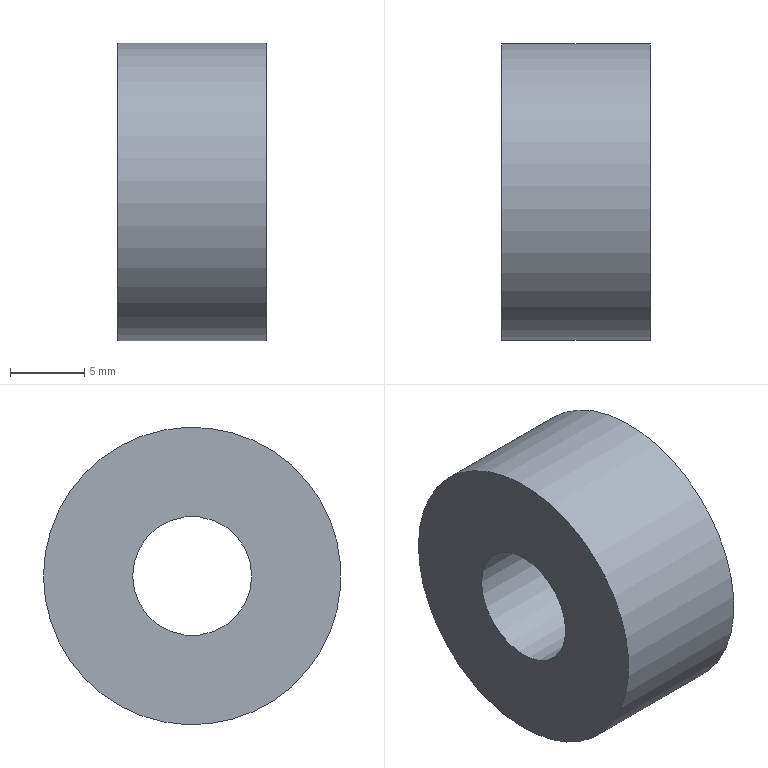Part | NX | features DATUM_CSYS 2, EXTRUDE 1, SKETCH 1 | 1 solid | 4 faces | box 10 x 20 x 20 mm | volume 2639 mm3 | cylinder 2 | plane 2 | commonest cylinder face diameters 8 x1 20 x1
STEP:
#1=CARTESIAN_POINT('',(10.,10.,0.));
#2=VERTEX_POINT('',#1);
#3=CARTESIAN_POINT('',(10.,0.,0.));
#4=DIRECTION('',(1.,0.,0.));
#5=DIRECTION('',(0.,1.,0.));
#6=AXIS2_PLACEMENT_3D('',#3,#4,#5);
#7=CIRCLE('',#6,10.);
#8=EDGE_CURVE('',#2,#2,#7,.T.);
#9=ORIENTED_EDGE('',*,*,#8,.F.);
#10=EDGE_LOOP('',(#9));
#11=FACE_BOUND('',#10,.T.);
#12=CARTESIAN_POINT('',(0.,10.,0.));
#13=VERTEX_POINT('',#12);
#14=CARTESIAN_POINT('',(0.,0.,0.));
#15=DIRECTION('',(1.,0.,0.));
#16=DIRECTION('',(0.,1.,0.));
#17=AXIS2_PLACEMENT_3D('',#14,#15,#16);
#18=CIRCLE('',#17,10.);
#19=EDGE_CURVE('',#13,#13,#18,.T.);
#20=ORIENTED_EDGE('',*,*,#19,.T.);
#21=EDGE_LOOP('',(#20));
#22=FACE_BOUND('',#21,.T.);
#23=CARTESIAN_POINT('',(10.,0.,0.));
#24=DIRECTION('',(-1.,0.,0.));
#25=DIRECTION('',(0.,0.,1.));
#26=AXIS2_PLACEMENT_3D('',#23,#24,#25);
#27=CYLINDRICAL_SURFACE('',#26,10.);
#28=ADVANCED_FACE('',(#11,#22),#27,.T.);
#29=CARTESIAN_POINT('',(10.,4.,0.));
#30=VERTEX_POINT('',#29);
#31=CARTESIAN_POINT('',(10.,0.,0.));
#32=DIRECTION('',(1.,0.,0.));
#33=DIRECTION('',(0.,1.,0.));
#34=AXIS2_PLACEMENT_3D('',#31,#32,#33);
#35=CIRCLE('',#34,4.);
#36=EDGE_CURVE('',#30,#30,#35,.T.);
#37=ORIENTED_EDGE('',*,*,#36,.T.);
#38=EDGE_LOOP('',(#37));
#39=FACE_BOUND('',#38,.T.);
#40=CARTESIAN_POINT('',(0.,4.,0.));
#41=VERTEX_POINT('',#40);
#42=CARTESIAN_POINT('',(0.,0.,0.));
#43=DIRECTION('',(1.,0.,0.));
#44=DIRECTION('',(0.,1.,0.));
#45=AXIS2_PLACEMENT_3D('',#42,#43,#44);
#46=CIRCLE('',#45,4.);
#47=EDGE_CURVE('',#41,#41,#46,.T.);
#48=ORIENTED_EDGE('',*,*,#47,.F.);
#49=EDGE_LOOP('',(#48));
#50=FACE_BOUND('',#49,.T.);
#51=CARTESIAN_POINT('',(10.,0.,0.));
#52=DIRECTION('',(-1.,0.,0.));
#53=DIRECTION('',(0.,0.,1.));
#54=AXIS2_PLACEMENT_3D('',#51,#52,#53);
#55=CYLINDRICAL_SURFACE('',#54,4.);
#56=ADVANCED_FACE('',(#39,#50),#55,.F.);
#57=ORIENTED_EDGE('',*,*,#8,.T.);
#58=EDGE_LOOP('',(#57));
#59=FACE_BOUND('',#58,.T.);
#60=ORIENTED_EDGE('',*,*,#36,.F.);
#61=EDGE_LOOP('',(#60));
#62=FACE_BOUND('',#61,.T.);
#63=CARTESIAN_POINT('',(10.,0.,0.));
#64=DIRECTION('',(1.,0.,0.));
#65=DIRECTION('',(0.,0.,-1.));
#66=AXIS2_PLACEMENT_3D('',#63,#64,#65);
#67=PLANE('',#66);
#68=ADVANCED_FACE('',(#59,#62),#67,.T.);
#69=ORIENTED_EDGE('',*,*,#19,.F.);
#70=EDGE_LOOP('',(#69));
#71=FACE_BOUND('',#70,.T.);
#72=ORIENTED_EDGE('',*,*,#47,.T.);
#73=EDGE_LOOP('',(#72));
#74=FACE_BOUND('',#73,.T.);
#75=CARTESIAN_POINT('',(0.,0.,0.));
#76=DIRECTION('',(1.,0.,0.));
#77=DIRECTION('',(0.,0.,-1.));
#78=AXIS2_PLACEMENT_3D('',#75,#76,#77);
#79=PLANE('',#78);
#80=ADVANCED_FACE('',(#71,#74),#79,.F.);
#81=CLOSED_SHELL('',(#28,#56,#68,#80));
#82=MANIFOLD_SOLID_BREP('',#81);
#83=(LENGTH_UNIT()NAMED_UNIT(*)SI_UNIT(.MILLI.,.METRE.));
#84=UNCERTAINTY_MEASURE_WITH_UNIT(LENGTH_MEASURE(0.00001),#83,'','');
#85=(NAMED_UNIT(*)PLANE_ANGLE_UNIT()SI_UNIT($,.RADIAN.));
#86=(NAMED_UNIT(*)SI_UNIT($,.STERADIAN.)SOLID_ANGLE_UNIT());
#87=(GEOMETRIC_REPRESENTATION_CONTEXT(3)GLOBAL_UNCERTAINTY_ASSIGNED_CONTEXT((#84))GLOBAL_UNIT_ASSIGNED_CONTEXT((#83,#85,#86))REPRESENTATION_CONTEXT('',''));
#88=ADVANCED_BREP_SHAPE_REPRESENTATION('',(#82),#87);